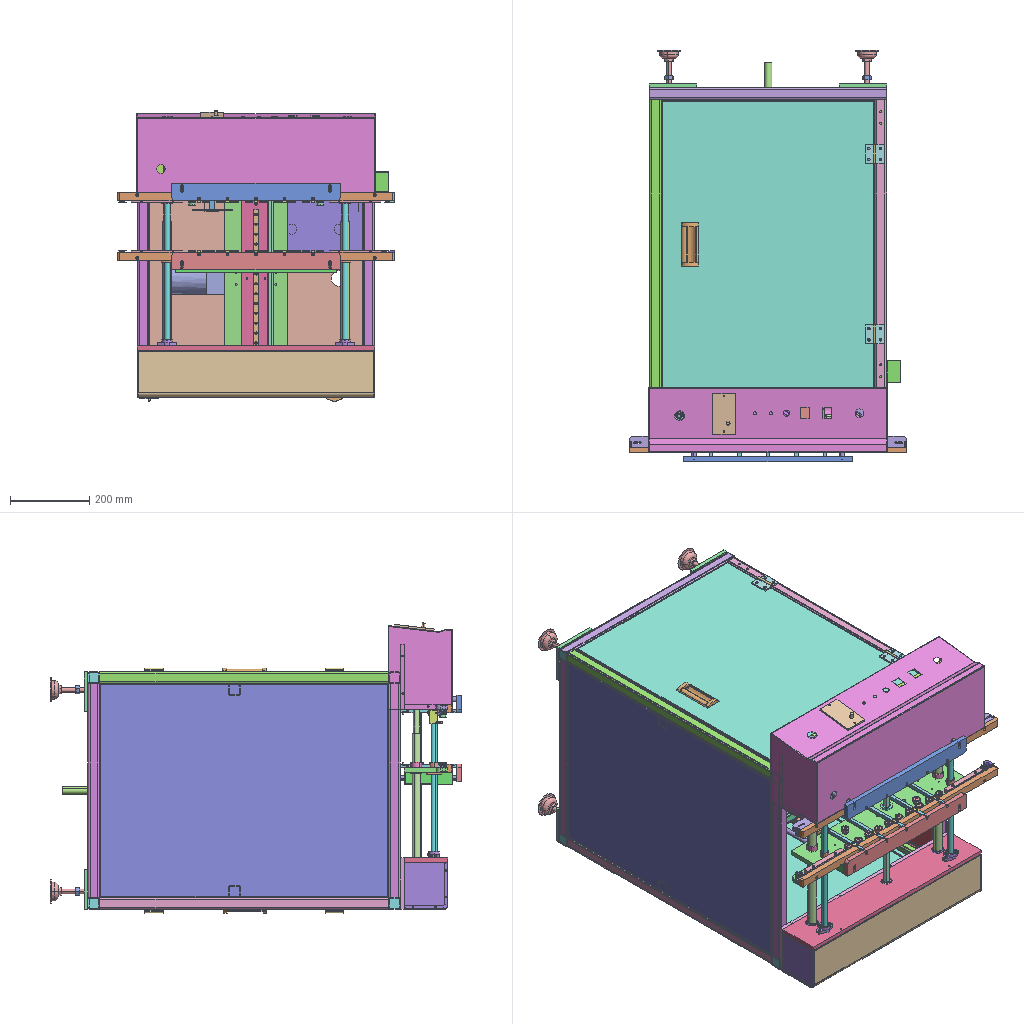Assembly | SolidWorks | 117 different items | 399 placed | box 700 x 1040 x 734 mm
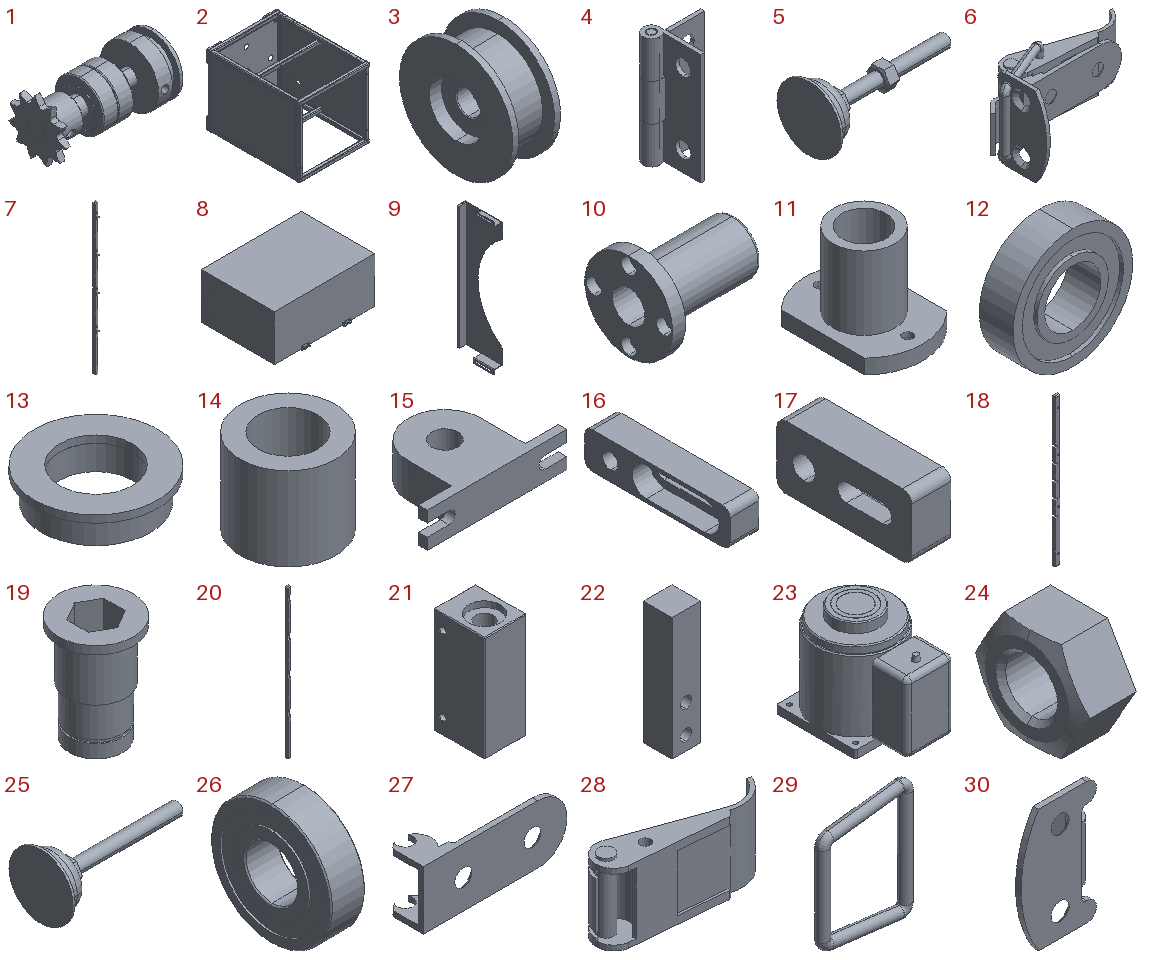Parts list (item | name | quantity | parent item | size | volume | features):
1 | (subassembly) | x22 | - | 38.5 x 19 x 19 mm | 5350 mm3 | -
2 | (subassembly) | x1 | - | 600 x 800 x 600 mm | 4319374 mm3 | -
3 | (subassembly) | x1 | - | 8 x 19 x 19 mm | 1286 mm3 | -
4 | (subassembly) | x2 | in 8 | 11.9 x 11.9 x 25 mm | 590.722 mm3 | -
5 | (subassembly) | x4 | - | 128 x 60 x 60 mm | 51221 mm3 | -
6 | (subassembly) | x2 | in 8 | 39.831 x 19.634 x 22 mm | 1988 mm3 | -
7 | (subassembly) | x10 | - | 8 x 12 x 450 mm | 28666 mm3 | -
8 | (subassembly) | x1 | - | 330 x 252.816 x 156.5 mm | 11874389 mm3 | -
9 | (subassembly) | x1 | - | 21.5 x 91 x 322 mm | 41867 mm3 | -
10 | - | x2 | - | 65 x 54 x 54 mm | 42042 mm3 | features LPattern 1, RevCut 1, Revolution 1
11 | - | x2 | - | 28 x 40 x 30 mm | 8237 mm3 | features ICE 2, Extrusion 1, HoleWzd 1
12 | - | x4 | - | 32 x 9 x 32 mm | 5125 mm3 | features Revolution 1
13 | - | x7 | - | 13.6 x 13.6 x 3.5 mm | 245.378 mm3 | features Extrusion 1, ICE 1
14 | - | x1 | - | 8 x 8 x 7 mm | 214.414 mm3 | features Extrusion 1
15 | - | x2 | - | 80 x 51 x 20 mm | 38253 mm3 | features Extrusion 1, ICE 1
16 | - | x3 | - | 8 x 40 x 10 mm | 1941 mm3 | features Fillet 2, ICE 2, Extrusion 1, HoleWzd 1
17 | - | x1 | - | 8.7 x 30 x 14 mm | 2717 mm3 | features ICE 2, Extrusion 1, Fillet 1, HoleWzd 1
18 | - | x2 | - | 20.5 x 15 x 700 mm | 182437 mm3 | features Chamfer 2, Extrusion 1, Fillet 1, HoleWzd 1, ICE 1
19 | - | x1 | - | 28 x 28 x 39.7 mm | 7720 mm3 | features ICE 5, Extrusion 1, RevCut 1
20 | - | x10 | in 7 | 8 x 8 x 450 mm | 26809 mm3 | features HoleWzd 3, ICE 2, Extrusion 1
21 | - | x4 | - | 28 x 34 x 70 mm | 55264 mm3 | features RevCut 7, ICE 2, Extrusion 1
22 | - | x1 | - | 8 x 8 x 35 mm | 2103 mm3 | features Extrusion 1, HoleWzd 1
23 | - | x2 | - | 80 x 115 x 116 mm | 570040 mm3 | features ICE 7, Fillet 2, 3DProfileFeature 1, Chamfer 1, Extrusion 1, HoleWzd 1
24 | - | x4 | in 5 | 10 x 21.939 x 19 mm | 2247 mm3 | features RefAxis 3, 3DProfileFeature 1, ICE 1, Revolution 1
25 | - | x4 | in 5 | 128 x 60 x 60 mm | 48974 mm3 | features RefAxis 9, 3DProfileFeature 3, ICE 1, Revolution 1
26 | - | x2 | - | 8 x 28 x 28 mm | 3855 mm3 | features RefAxis 3, 3DProfileFeature 1, Revolution 1
27 | - | x2 | in 6 | 27 x 6.688 x 11 mm | 304.183 mm3 | features RefAxis 3, ICE 2, RevCut 2, 3DProfileFeature 1, Extrusion 1
28 | - | x2 | in 6 | 30 x 8.531 x 15 mm | 1203 mm3 | features ICE 6, RefAxis 6, 3DProfileFeature 2, Extrusion 1
29 | - | x2 | in 6 | 16.763 x 2 x 21.5 mm | 200.249 mm3 | features RefAxis 6, Revolution 4, ICE 3, 3DProfileFeature 2, Extrusion 1
30 | - | x2 | in 6 | 13.5 x 6.5 x 22 mm | 280.062 mm3 | features RefAxis 3, ICE 2, RevCut 2, 3DProfileFeature 1, Extrusion 1
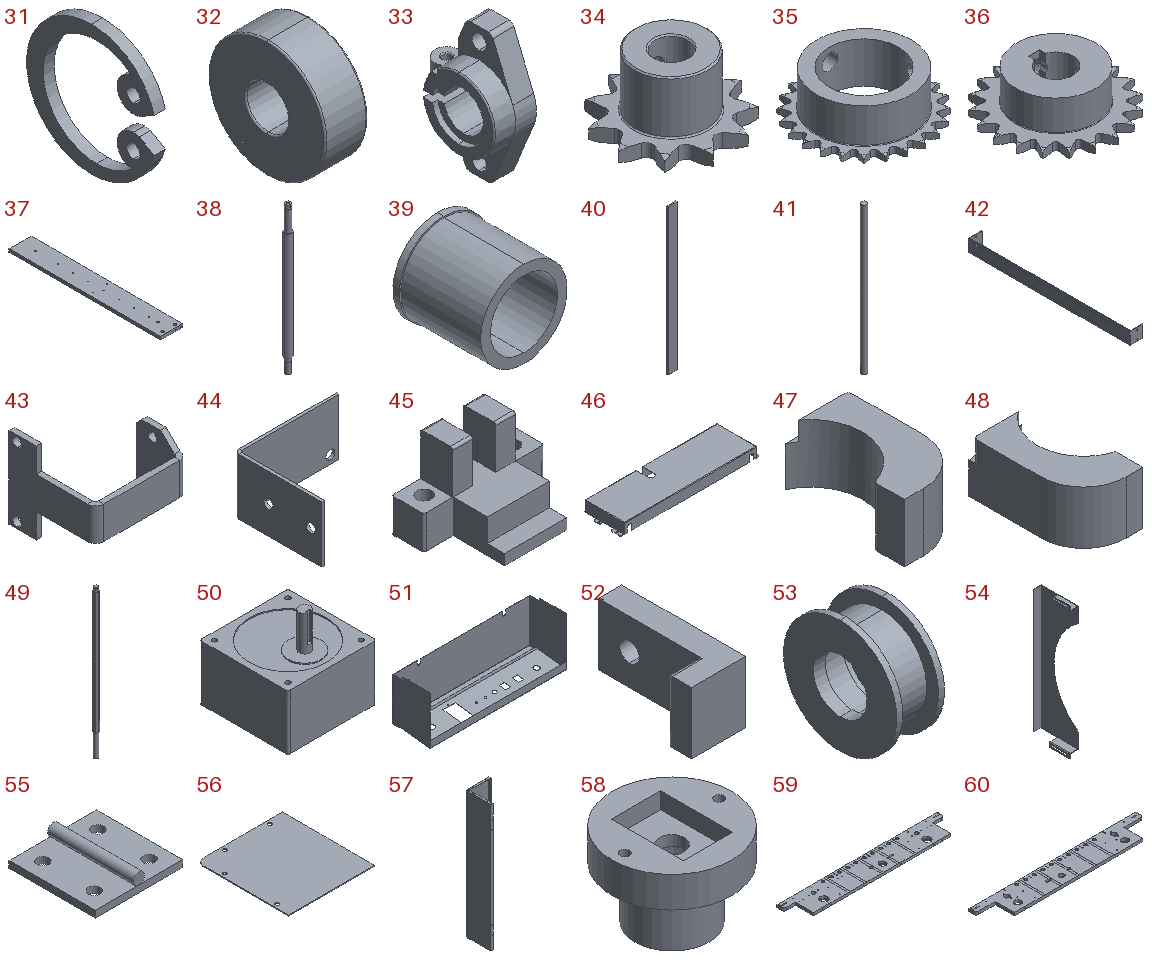31 | - | x1 | in 3 | 1 x 11.586 x 11.8 mm | 42.993 mm3 | features RefAxis 3, 3DProfileFeature 1, Extrusion 1
32 | - | x1 | in 3 | 4 x 11 x 11 mm | 327.696 mm3 | features RefAxis 6, 3DProfileFeature 2, Revolution 1
33 | - | x4 | - | 16 x 31 x 50 mm | 9253 mm3 | features ICE 5, RefAxis 3, RevCut 3, 3DProfileFeature 1, Extrusion 1, Revolution 1
34 | - | x22 | in 1 | 18.807 x 18.615 x 10 mm | 909.903 mm3 | features RevCut 2, ICE 1, Revolution 1
35 | - | x1 | - | 39 x 39 x 13 mm | 4619 mm3 | features ICE 3, RevCut 2, Revolution 1
36 | - | x3 | - | 44 x 44 x 13.5 mm | 8028 mm3 | features ICE 3, RevCut 2, Revolution 1
37 | - | x1 | - | 72 x 496 x 10 mm | 354695 mm3 | features HoleWzd 6, Extrusion 1
38 | - | x2 | - | 21 x 21 x 431 mm | 129224 mm3 | features ICE 5, HoleWzd 2, 3DProfileFeature 1, Extrusion 1
39 | - | x2 | - | 28 x 27 x 28 mm | 6194 mm3 | features Revolution 1
40 | - | x1 | in 9 | 18 x 3 x 300 mm | 16200 mm3 | features Extrusion 1
41 | - | x1 | - | 15 x 15 x 430 mm | 75987 mm3 | features Extrusion 1
42 | - | x1 | - | 31.5 x 395 x 30 mm | 22778 mm3 | features ICE 3, FlatPattern 1, SMBaseFlange 1, SheetMetal 1
43 | - | x1 | - | 34 x 32 x 30 mm | 2372 mm3 | features ICE 5, Chamfer 1, FlatPattern 1, SMBaseFlange 1, SheetMetal 1
44 | - | x3 | - | 36 x 31 x 20 mm | 1279 mm3 | features ICE 2, FlatPattern 1, SMBaseFlange 1, SheetMetal 1
45 | - | x2 | - | 26.2 x 18.3 x 16.6 mm | 2634 mm3 | features ICE 5, Fillet 2, Extrusion 1, MirrorPattern 1
46 | - | x1 | - | 427 x 122 x 32 mm | 79185 mm3 | features Cut 3, EdgeFlange 3, Fillet 1, FlatPattern 1, ICE 1, SMBaseFlange 1, SheetMetal 1
47 | - | x1 | - | 14 x 27 x 12.5 mm | 2830 mm3 | features Fillet 3, Extrusion 1, HoleWzd 1, ICE 1
48 | - | x1 | - | 14 x 27 x 12.5 mm | 2831 mm3 | features Fillet 2, ICE 2, Extrusion 1, HoleWzd 1, MirrorPattern 1
49 | - | x1 | - | 14 x 16.166 x 456 mm | 72301 mm3 | features ICE 3, Fillet 2, Extrusion 1, RevCut 1
50 | - | x2 | - | 80 x 80 x 82 mm | 314622 mm3 | features ICE 5, 3DProfileFeature 1, Extrusion 1, Fillet 1, HoleWzd 1
51 | - | x1 | - | 602 x 163.116 x 210.993 mm | 271035 mm3 | features ICE 6, Cut 3, Fillet 3, ExtruThin 1, MirrorPattern 1
52 | - | x40 | in 7 | 7 x 16 x 8 mm | 464.439 mm3 | features Extrusion 1, Fillet 1, HoleWzd 1
53 | - | x4 | in 3 | 8 x 19 x 19 mm | 915.586 mm3 | features RefAxis 12, 3DProfileFeature 4, Revolution 1
54 | - | x1 | in 9 | 21.5 x 91 x 322 mm | 25667 mm3 | features ICE 3, EdgeFlange 2, FlatPattern 1, SMBaseFlange 1, SheetMetal 1
55 | - | x4 | - | 48 x 47 x 9.7 mm | 9200 mm3 | features Extrusion 1, ICE 1
56 | - | x2 | - | 110 x 118 x 1 mm | 12895 mm3 | features Cut 1, FlatPattern 1, SMBaseFlange 1, SheetMetal 1
57 | - | x1 | - | 110 x 118 x 598 mm | 147295 mm3 | features EdgeFlange 3, ICE 2, FlatPattern 1, HoleWzd 1, SMBaseFlange 1, SheetMetal 1
58 | - | x1 | - | 58 x 58 x 40 mm | 46736 mm3 | features ICE 3, Extrusion 1, HoleWzd 1
59 | - | x1 | - | 700 x 110 x 12 mm | 766656 mm3 | features HoleWzd 15, ICE 11, Cut 1, Extrusion 1, Fillet 1
60 | - | x1 | - | 700 x 110 x 12 mm | 712191 mm3 | features HoleWzd 12, ICE 7, Extrusion 1, Fillet 1, LPattern 1
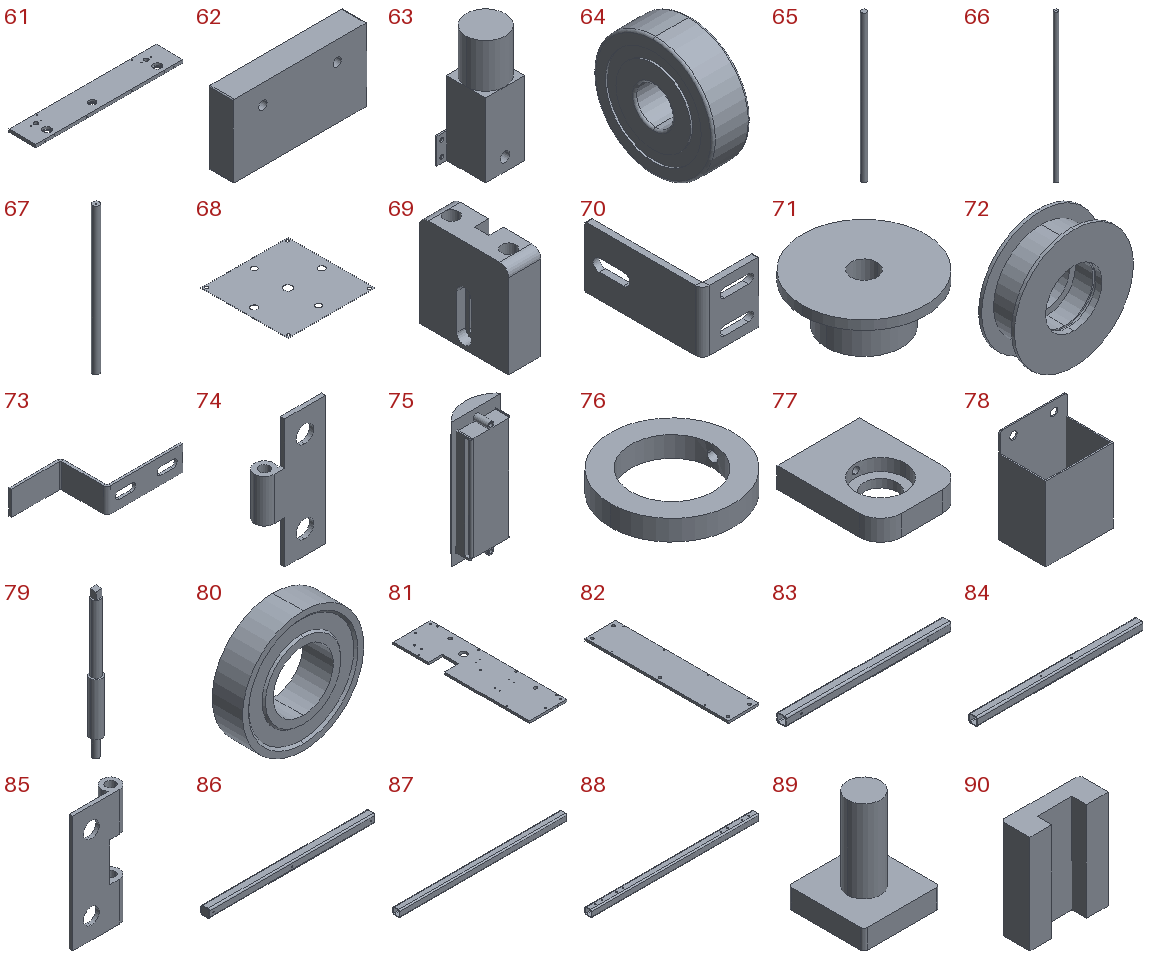61 | - | x1 | - | 600 x 110 x 12 mm | 762368 mm3 | features ICE 5, HoleWzd 4, Extrusion 1
62 | - | x1 | - | 72 x 13 x 39 mm | 36088 mm3 | features Extrusion 1, Fillet 1, ICE 1
63 | - | x1 | - | 120 x 83 x 241 mm | 1411191 mm3 | features ICE 4, Extrusion 1
64 | - | x44 | in 1 | 5 x 16 x 16 mm | 879.517 mm3 | features Revolution 1
65 | - | x2 | - | 15 x 15 x 430 mm | 75987 mm3 | features Extrusion 1
66 | - | x4 | - | 12 x 12 x 448 mm | 50405 mm3 | features HoleWzd 2, Extrusion 1
67 | - | x2 | - | 20 x 20 x 445 mm | 139374 mm3 | features HoleWzd 2, Extrusion 1
68 | - | x1 | in 2 | 540 x 540 x 1 mm | 284181 mm3 | features Cut 2, ICE 2, Extrusion 1
69 | - | x2 | - | 18 x 50 x 52 mm | 37362 mm3 | features ICE 2, Extrusion 1, Fillet 1, HoleWzd 1
70 | - | x1 | - | 28 x 58 x 30 mm | 6672 mm3 | features ICE 2, Fillet 1, FlatPattern 1, SMBaseFlange 1, SheetMetal 1
71 | - | x1 | - | 37.5 x 37.5 x 14.8 mm | 7334 mm3 | features Extrusion 1, ICE 1
72 | - | x4 | - | 40 x 12 x 40 mm | 7443 mm3 | features Revolution 1
73 | - | x1 | - | 51 x 20 x 10 mm | 643.331 mm3 | features EdgeFlange 1, FlatPattern 1, ICE 1, SMBaseFlange 1, SheetMetal 1
74 | - | x2 | in 4 | 11.9 x 3.8 x 25 mm | 218.697 mm3 | features ICE 3, RefAxis 3, 3DProfileFeature 1, Extrusion 1
75 | - | x2 | - | 43.5 x 22.46 x 110 mm | 28533 mm3 | features ICE 3, Extrusion 1, Fillet 1, MirrorPattern 1
76 | - | x1 | - | 30 x 30 x 5 mm | 1939 mm3 | features 3DProfileFeature 1, Extrusion 1, HoleWzd 1
77 | - | x1 | - | 40 x 50 x 10 mm | 15721 mm3 | features HoleWzd 2, ICE 2, Extrusion 1, Fillet 1
78 | - | x1 | - | 50 x 35 x 70 mm | 11415 mm3 | features ICE 3, Extrusion 1, Fillet 1
79 | - | x1 | - | 16 x 16 x 196 mm | 26092 mm3 | features ICE 3, Extrusion 1
80 | - | x1 | - | 24 x 6 x 24 mm | 1915 mm3 | features Revolution 1
81 | - | x1 | - | 165 x 600 x 10 mm | 927945 mm3 | features HoleWzd 8, Cut 2, Extrusion 1, ICE 1
82 | - | x1 | - | 130 x 600 x 10 mm | 774782 mm3 | features HoleWzd 3, Extrusion 1
83 | - | x4 | in 2 | 540 x 30 x 30 mm | 144334 mm3 | features HoleWzd 2, 3DProfileFeature 1, WeldMemberFeat 1, WeldmentFeature 1
84 | - | x2 | in 2 | 598 x 30 x 30 mm | 159852 mm3 | features 3DProfileFeature 1, HoleWzd 1, WeldMemberFeat 1, WeldmentFeature 1
85 | - | x2 | in 4 | 11.9 x 3.8 x 25 mm | 293.72 mm3 | features ICE 3, RefAxis 3, 3DProfileFeature 1, Extrusion 1
86 | - | x4 | in 2 | 600 x 30 x 30 mm | 162072 mm3 | features ICE 2, 3DProfileFeature 1, HoleWzd 1, WeldMemberFeat 1, WeldmentFeature 1
87 | - | x2 | in 2 | 730 x 30 x 30 mm | 195313 mm3 | features 3DProfileFeature 1, WeldMemberFeat 1, WeldmentFeature 1
88 | - | x2 | in 2 | 730 x 30 x 30 mm | 194616 mm3 | features HoleWzd 2, 3DProfileFeature 1, WeldMemberFeat 1, WeldmentFeature 1
89 | - | x1 | - | 23 x 23 x 31 mm | 5132 mm3 | features Extrusion 1, Fillet 1, ICE 1
90 | - | x1 | - | 27 x 10 x 34 mm | 6954 mm3 | features Chamfer 1, Extrusion 1, HoleWzd 1
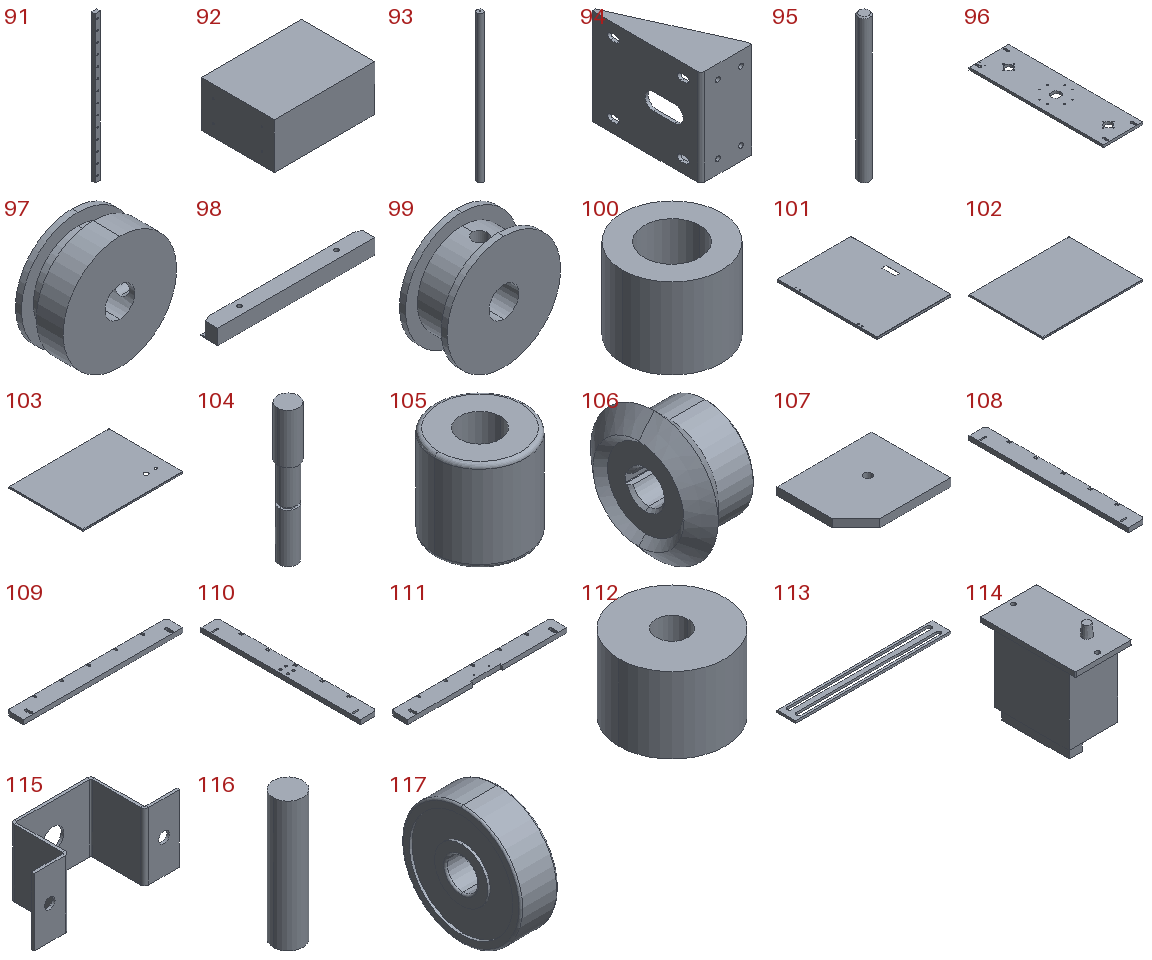91 | - | x1 | - | 12 x 8 x 350 mm | 31582 mm3 | features Chamfer 2, Extrusion 1, HoleWzd 1, LPattern 1
92 | - | x1 | in 8 | 330 x 240 x 150 mm | 11869232 mm3 | features Cut 2, Extrusion 1
93 | - | x1 | - | 20 x 20 x 500 mm | 156724 mm3 | features HoleWzd 2, Extrusion 1
94 | - | x1 | - | 48 x 103 x 91 mm | 51216 mm3 | features ICE 4, Cut 1, FlatPattern 1, SMBaseFlange 1, SheetMetal 1
95 | - | x2 | in 4 | 2 x 2 x 25 mm | 78.305 mm3 | features RefAxis 3, 3DProfileFeature 1, Revolution 1
96 | - | x1 | - | 160 x 540 x 10 mm | 829534 mm3 | features HoleWzd 7, ICE 4, Extrusion 1
97 | - | x22 | in 1 | 19 x 8 x 19 mm | 1809 mm3 | features 3DProfileFeature 1, HoleWzd 1, Revolution 1
98 | - | x4 | - | 130 x 14 x 12.5 mm | 20035 mm3 | features Chamfer 2, Extrusion 1, HoleWzd 1, ICE 1
99 | - | x2 | - | 19 x 8 x 19 mm | 1445 mm3 | features 3DProfileFeature 1, HoleWzd 1, Revolution 1
100 | - | x4 | - | 8 x 8 x 6.5 mm | 223.348 mm3 | features Extrusion 1, ICE 1
101 | - | x2 | - | 539 x 728 x 18 mm | 690643 mm3 | features EdgeFlange 5, Cut 1, FlatPattern 1, ICE 1, SMBaseFlange 1, SheetMetal 1, WeldmentFeature 1
102 | - | x1 | in 2 | 729.5 x 540 x 11.5 mm | 626320 mm3 | features EdgeFlange 3, FlatPattern 1, SMBaseFlange 1, SMMiteredFlange 1, SheetMetal 1
103 | - | x1 | in 2 | 729.5 x 540 x 11.5 mm | 624958 mm3 | features EdgeFlange 3, FlatPattern 1, ICE 1, SMBaseFlange 1, SMMiteredFlange 1, SheetMetal 1
104 | - | x22 | in 1 | 6 x 6 x 38.5 mm | 871.949 mm3 | features Extrusion 1, ICE 1, RevCut 1
105 | - | x2 | - | 45 x 45 x 45 mm | 57194 mm3 | features Extrusion 1, Fillet 1, ICE 1
106 | - | x6 | - | 21.26 x 39.62 x 39.62 mm | 14366 mm3 | features RefAxis 12, 3DProfileFeature 4, RevCut 2, ICE 1, Revolution 1
107 | - | x4 | in 2 | 120 x 100 x 10 mm | 114683 mm3 | features Extrusion 1, HoleWzd 1
108 | - | x1 | - | 44 x 425 x 12 mm | 219705 mm3 | features ICE 5, Extrusion 1, Fillet 1, LPattern 1
109 | - | x1 | - | 425 x 44 x 12 mm | 219705 mm3 | features ICE 5, Extrusion 1, Fillet 1, LPattern 1
110 | - | x1 | - | 44 x 425 x 12 mm | 219009 mm3 | features ICE 5, Extrusion 1, Fillet 1, HoleWzd 1, LPattern 1
111 | - | x1 | - | 425 x 44 x 12 mm | 214700 mm3 | features ICE 6, Extrusion 1, Fillet 1, HoleWzd 1, LPattern 1
112 | - | x4 | - | 14 x 14 x 10 mm | 1401 mm3 | features Extrusion 1, HoleWzd 1
113 | - | x1 | - | 100 x 12 x 1.5 mm | 968.794 mm3 | features Extrusion 1
114 | - | x1 | - | 60 x 102 x 104 mm | 355291 mm3 | features ICE 3, Extrusion 1, Fillet 1
115 | - | x1 | - | 54 x 21 x 25 mm | 2232 mm3 | features ICE 2, FlatPattern 1, SMBaseFlange 1, SheetMetal 1
116 | - | x1 | - | 8 x 8 x 35 mm | 1759 mm3 | features Extrusion 1
117 | - | x4 | - | 6 x 19 x 19 mm | 1455 mm3 | features RefAxis 6, 3DProfileFeature 2, Revolution 1
Mates (type | each side: item.copy, entity, surface, feature), first 403 of 428 lines:
In the top assembly
Coincident | 101.1 face plane Base-Flange 1 | 75.1 face plane Boss-Extrude 1
Coincident | 101.1 face plane Cut-Extrude 1 | 75.1 face plane Boss-Extrude 1
Coincident | 101.1 face plane Cut-Extrude 1 | 75.1 face plane Cut-Extrude 11
Coincident | 101.2 face plane Base-Flange 1 | 75.2 face plane Boss-Extrude 1
Coincident | 101.2 face plane Cut-Extrude 1 | 75.2 face plane Boss-Extrude 1
Coincident | 101.2 face plane Cut-Extrude 1 | 75.2 face plane Cut-Extrude 11
Coincident | 82.1 face plane Boss-Extrude 1 | 59.1 face plane Boss-Extrude 1
Coincident | 59.1 face plane Boss-Extrude 1 | 60.1 face plane Boss-Extrude 1
Coincident | 60.1 face plane Boss-Extrude 1 | 61.1 face plane Boss-Extrude 1
Coincident | 82.1 face plane Boss-Extrude 1 | 61.1 face plane Boss-Extrude 1 | 2 times
Concentric | 60.1 face cylinder Cut-Extrude 2 | 38.1 face cylinder Boss-Extrude 3
Concentric | 59.1 face cylinder Cut-Extrude 3 | 12.1 face cylinder Revolve 1
Coincident | 59.1 face plane Boss-Extrude 1 | 12.1 face plane Revolve 1
Concentric | 59.1 face cylinder Cut-Extrude 3 | 12.2 face cylinder Revolve 1
Coincident | 59.1 face plane Boss-Extrude 1 | 12.2 face plane Revolve 1
Concentric | 38.1 face cylinder Boss-Extrude 3 | 12.3 face cylinder Revolve 1
Coincident | 61.1 face plane Boss-Extrude 1 | 12.3 face plane Revolve 1
Concentric | 61.1 face cylinder Cut-Extrude 2 | 12.4 face cylinder Revolve 1
Coincident | 61.1 face plane Boss-Extrude 1 | 12.4 face plane Revolve 1
Concentric | 60.1 face cylinder Cut-Extrude 2 | 65.1 face cylinder Boss-Extrude 1
Concentric | 60.1 face cylinder Cut-Extrude 2 | 11.1 face cylinder Boss-Extrude 1
Concentric | 65.1 face cylinder Boss-Extrude 1 | 11.2 face cylinder Boss-Extrude 1
Concentric | 12.1 face cylinder Revolve 1 | 38.2 face cylinder Boss-Extrude 1
Concentric | 11.1 face cylinder Boss-Extrude 1 | 65.2 face cylinder Boss-Extrude 1
Coincident | 60.1 face plane Boss-Extrude 1 | 11.1 face plane Boss-Extrude 3
Coincident | 60.1 face plane Boss-Extrude 1 | 11.2 face plane Boss-Extrude 3
Coincident | 61.1 face plane Boss-Extrude 1 | 38.1 face plane Boss-Extrude 3
Concentric | 38.1 face cylinder Boss-Extrude 5 | 36.1 face cylinder Revolve 1
Concentric | 38.2 face cylinder Boss-Extrude 5 | 36.2 face cylinder Revolve 1
Coincident | 61.1 face plane Boss-Extrude 1 | 33.1 face plane Boss-Extrude 1
Concentric | 65.1 face cylinder Boss-Extrude 1 | 33.1 face cylinder Cut-Revolve 1
Coincident | 59.1 face plane Boss-Extrude 1 | 33.2 face plane Boss-Extrude 1
Concentric | 65.1 face cylinder Boss-Extrude 1 | 33.2 face cylinder Cut-Revolve 1
Concentric | 65.2 face cylinder Boss-Extrude 1 | 33.3 face cylinder Cut-Revolve 1
Coincident | 61.1 face plane Boss-Extrude 1 | 33.3 face plane Boss-Extrude 1
Concentric | 65.2 face cylinder Boss-Extrude 1 | 33.4 face cylinder Cut-Revolve 1
Coincident | 59.1 face plane Boss-Extrude 1 | 33.4 face plane Boss-Extrude 1
Concentric | 59.1 face | assembly face | 2 times
Coincident | 59.1 face plane Boss-Extrude 1 | assembly face
Parallel | 61.1 face plane Boss-Extrude 1 | 33.3 face plane Cut-Extrude 2
Parallel | 61.1 face plane Boss-Extrude 1 | 33.1 face plane Cut-Extrude 2
Parallel | 59.1 face plane Boss-Extrude 1 | 33.2 face plane Cut-Extrude 2
Parallel | 59.1 face plane Boss-Extrude 1 | 33.4 face plane Cut-Extrude 2
Concentric | 60.1 face cylinder Cut-Extrude 5 | 53.1 face cylinder Revolve 1
Concentric | 59.1 face cylinder Cut-Extrude 6 | 53.2 face cylinder Revolve 1
Coincident | 60.1 face plane Boss-Extrude 1 | 19.1 face plane Cut-Extrude 1
Coincident | 59.1 face plane Boss-Extrude 1 | 18.1 face plane Boss-Extrude 1 | 3 times
Coincident | 66.1 face plane Boss-Extrude 1 | 66.2 face plane Boss-Extrude 1
Coincident | 66.1 face plane Boss-Extrude 1 | 66.3 face plane Boss-Extrude 1
Coincident | 66.2 face plane Boss-Extrude 1 | 66.4 face plane Boss-Extrude 1
Concentric | 10.1 face cylinder Revolve 1 | 67.1 face cylinder Boss-Extrude 1
Concentric | 10.2 face cylinder Revolve 1 | 67.2 face cylinder Boss-Extrude 1
Concentric | 49.1 face cylinder Boss-Extrude 2 | 106.1 face cylinder Revolve 1
Coincident | 94.1 face plane Base-Flange 1 | 50.1 face plane Boss-Extrude 1
Parallel | 94.1 face plane Base-Flange 1 | 50.1 face plane Boss-Extrude 1
Concentric | 106.2 face cylinder Revolve 1 | 50.1 face cylinder Boss-Extrude 3
Parallel | 81.1 face plane Boss-Extrude 1 | 94.1 face plane Boss-Extrude 2 | 2 times
Coincident | 106.2 face plane Revolve 1 | 50.1 face plane Boss-Extrude 3
Width | 94.1 face plane Boss-Extrude 2 | 94.1 face plane Boss-Extrude 1 | 50.1 face plane Boss-Extrude 1 | 50.1 face plane Boss-Extrude 1
Coincident | 60.1 face plane Boss-Extrude 1 | assembly face
Coincident | 60.1 face plane Boss-Extrude 1 | 18.2 face plane Boss-Extrude 1 | 3 times
Concentric | 49.1 face cylinder Boss-Extrude 2 | 36.3 face cylinder Revolve 1
Concentric | 60.1 face cylinder Cut-Extrude 2 | 35.1 face cylinder Revolve 1
Concentric | 96.1 face cylinder Cut-Extrude 1 | 10.2 face cylinder Revolve 1
Concentric | 96.1 face cylinder Cut-Extrude 1 | 10.1 face cylinder Revolve 1
Parallel | 96.1 face plane Boss-Extrude 1 | 37.1 face plane Boss-Extrude 1
Coincident | 96.1 face plane Boss-Extrude 1 | 10.1 face plane Revolve 1
Coincident | 96.1 face plane Boss-Extrude 1 | 10.2 face plane Revolve 1
Coincident | 37.1 face plane Boss-Extrude 1 | 67.2 face plane Boss-Extrude 1
Coincident | 37.1 face plane Boss-Extrude 1 | 67.1 face plane Boss-Extrude 1
Width | 96.1 face plane Boss-Extrude 1 | 96.1 face plane Boss-Extrude 1 | 37.1 face plane Boss-Extrude 1 | 37.1 face plane Boss-Extrude 1
Coincident | 37.1 face plane Boss-Extrude 1 | 73.1 face plane Base-Flange 1 | 3 times
Coincident | 81.1 face plane Boss-Extrude 1 | 59.1 face plane Boss-Extrude 1 | 2 times
Coincident | 82.1 face plane Boss-Extrude 1 | 57.1 face plane Edge-Flange 1
Coincident | 61.1 face plane Boss-Extrude 1 | 57.1 face plane Edge-Flange 1
Coincident | 57.1 face plane Edge-Flange 2 | 56.1 face plane Base-Flange 1
Coincident | 57.1 face plane Base-Flange 1 | 56.1 face plane Base-Flange 1 | 2 times
Coincident | 57.1 face plane Edge-Flange 3 | 56.2 face plane Base-Flange 1
Coincident | 57.1 face plane Base-Flange 1 | 56.2 face plane Base-Flange 1 | 2 times
Concentric | 53.2 face cylinder Revolve 1 | 100.1 face cylinder Boss-Extrude 1
Coincident | 59.1 face plane Boss-Extrude 1 | 100.1 face plane Boss-Extrude 1
Coincident | 59.1 face plane Boss-Extrude 1 | 44.1 face plane Base-Flange 1
Coincident | 59.1 face plane Boss-Extrude 1 | 44.2 face plane Base-Flange 1
Coincident | 96.1 face plane Boss-Extrude 1 | 42.1 face plane Base-Flange 1 | 2 times
Concentric | 80.1 face cylinder Revolve 1 | 77.1 face cylinder Cut-Extrude 1
Coincident | 80.1 face plane Revolve 1 | 77.1 face plane Boss-Extrude 1
Concentric | 12.1 face cylinder Revolve 1 | 80.1 face cylinder Revolve 1
Concentric | 80.1 face cylinder Revolve 1 | 79.1 face cylinder Boss-Extrude 3
DistanceDim | 77.1 face plane Boss-Extrude 1 | 81.1 face plane Boss-Extrude 1
DistanceDim | 12.1 face plane Revolve 1 | 79.1 face plane Boss-Extrude 3
Concentric | 117.1 face cylinder Revolve 1 | 72.1 face cylinder Revolve 1
Coincident | 117.1 face plane Revolve 1 | 72.1 face plane Revolve 1
Concentric | 72.1 face cylinder Revolve 1 | 112.1 face cylinder Boss-Extrude 1
Coincident | 60.1 face plane Boss-Extrude 1 | 112.1 face plane Boss-Extrude 1
Coincident | 117.1 face plane Revolve 1 | 112.1 face plane Boss-Extrude 1
Concentric | 117.2 face cylinder Revolve 1 | 112.2 face cylinder Boss-Extrude 1
Coincident | 117.2 face plane Revolve 1 | 112.2 face plane Boss-Extrude 1
Concentric | 117.2 face cylinder Revolve 1 | 72.2 face cylinder Revolve 1
Coincident | 60.1 face plane Boss-Extrude 1 | 112.2 face plane Boss-Extrude 1
Concentric | 117.3 face cylinder Revolve 1 | 112.3 face cylinder Boss-Extrude 1
Concentric | 117.3 face cylinder Revolve 1 | 72.3 face cylinder Revolve 1
Coincident | 117.3 face plane Revolve 1 | 72.3 face plane Revolve 1
Coincident | 117.3 face plane Revolve 1 | 112.3 face plane Boss-Extrude 1
Coincident | 59.1 face plane Boss-Extrude 1 | 112.3 face plane Boss-Extrude 1
Concentric | 112.4 face cylinder Boss-Extrude 1 | 72.4 face cylinder Revolve 1
Coincident | 117.2 face plane Revolve 1 | 72.2 face plane Revolve 1
Concentric | 117.4 face cylinder Revolve 1 | 112.4 face cylinder Boss-Extrude 1
Coincident | 117.4 face plane Revolve 1 | 112.4 face plane Boss-Extrude 1
Coincident | 117.4 face plane Revolve 1 | 72.4 face plane Revolve 1
Concentric | 81.1 face cylinder M4 Tapped Hole 1 | 94.1 face cylinder Cut-Extrude 2
DistanceDim | 57.1 face plane Edge-Flange 2 | 82.1 face plane Boss-Extrude 1
Coincident | 59.1 face plane Boss-Extrude 1 | 100.2 face plane Boss-Extrude 1
Concentric | 60.1 face cylinder Cut-Extrude 5 | 100.3 face cylinder Cut-Extrude 1
Coincident | 60.1 face plane Boss-Extrude 1 | 100.3 face plane Boss-Extrude 1
Coincident | 60.1 face plane Boss-Extrude 1 | 46.1 face plane Edge-Flange 1
Width | 60.1 face plane Boss-Extrude 1 | 60.1 face plane Boss-Extrude 1 | 46.1 face plane Edge-Flange 2 | 46.1 face plane Edge-Flange 2
Coincident | 60.1 face plane Boss-Extrude 1 | 46.1 face plane Edge-Flange 3
Concentric | 96.1 face cylinder M5 Tapped Hole 1 | 10.1 face cylinder LPattern 1
Concentric | 96.1 face cylinder M5 Tapped Hole 2 | 10.2 face cylinder LPattern 1
Coincident | 42.1 face plane Base-Flange 1 | 45.1 face plane Boss-Extrude 1
DistanceDim | 45.1 face plane Boss-Extrude 1 | 42.1 face plane Base-Flange 1
DistanceDim | 45.1 face plane Boss-Extrude 1 | 73.1 face plane Edge-Flange 1
Coincident | 42.1 face plane Base-Flange 1 | 45.2 face plane Boss-Extrude 1
Coincident | 45.1 face plane Boss-Extrude 1 | 45.2 face plane Boss-Extrude 1
Coincident | 66.2 face plane Boss-Extrude 1 | 108.1 face plane Boss-Extrude 1
Coincident | 66.4 face plane Boss-Extrude 1 | 109.1 face plane Boss-Extrude 1
Width | 59.1 face plane Boss-Extrude 1 | 59.1 face plane Boss-Extrude 1 | 109.1 face plane Boss-Extrude 1 | 109.1 face plane Boss-Extrude 1
Width | 60.1 face plane Boss-Extrude 1 | 60.1 face plane Boss-Extrude 1 | 108.1 face plane Boss-Extrude 1 | 108.1 face plane Boss-Extrude 1
Width | 59.1 face plane Boss-Extrude 1 | 59.1 face plane Boss-Extrude 1 | 111.1 face plane Boss-Extrude 1 | 111.1 face plane Boss-Extrude 1
Coincident | 59.1 face plane Boss-Extrude 1 | 98.1 face plane Boss-Extrude 1
Parallel | 18.1 face plane Boss-Extrude 1 | 98.1 face plane Boss-Extrude 1
DistanceDim | 98.1 face plane Boss-Extrude 1 | 59.1 face plane Boss-Extrude 1
Coincident | 60.1 face plane Boss-Extrude 1 | 100.4 face plane Boss-Extrude 1
Coincident | 97.1 face plane Revolve 1 | 53.3 face plane Revolve 1
Coincident | 60.1 face plane Boss-Extrude 1 | 98.2 face plane Boss-Extrude 1
DistanceDim | 98.2 face plane Boss-Extrude 1 | 60.1 face plane Boss-Extrude 1
Tangent | 53.1 face cylinder Revolve 1 | 98.2 face plane Cut-Extrude 1
Coincident | 59.1 face plane Boss-Extrude 1 | 98.3 face plane Boss-Extrude 1
DistanceDim | 98.3 face plane Boss-Extrude 1 | 59.1 face plane Boss-Extrude 1
Tangent | 53.4 face cylinder Revolve 1 | 98.3 face plane Cut-Extrude 1
Coincident | 60.1 face plane Boss-Extrude 1 | 98.4 face plane Boss-Extrude 1
DistanceDim | 98.4 face plane Boss-Extrude 1 | 60.1 face plane Boss-Extrude 1
Tangent | 53.3 face cylinder Revolve 1 | 98.4 face plane Cut-Extrude 1
Concentric | 60.1 face cylinder  Drill Hole Size by Socket Head Cap Screw Type 1 | 72.1 face cylinder Revolve 1
Concentric | 60.1 face cylinder Cut-Extrude 7 | 117.2 face cylinder Revolve 1
Concentric | 59.1 face cylinder  Drill Hole Size by Socket Head Cap Screw Type 2 | 117.3 face cylinder Revolve 1
Concentric | 59.1 face cylinder Cut-Extrude 9 | 117.4 face cylinder Revolve 1
Coincident | 59.1 face plane Boss-Extrude 1 | 112.4 face plane Boss-Extrude 1
Width | 36.3 face plane Revolve 1 | 36.3 face plane Revolve 1 | 72.4 face plane Revolve 1 | 72.4 face plane Revolve 1
DistanceDim | 18.1 face plane Boss-Extrude 1 | 44.1 face plane Base-Flange 1
DistanceDim | 18.1 face plane Boss-Extrude 1 | 44.2 face plane Base-Flange 1
Coincident | 59.1 face plane Boss-Extrude 1 | 44.3 face plane Base-Flange 1 | 2 times
DistanceDim | 18.1 face plane Boss-Extrude 1 | 44.3 face plane Base-Flange 1
DistanceDim | 44.2 face plane Base-Flange 1 | 59.1 face plane Boss-Extrude 1
DistanceDim | 44.1 face plane Base-Flange 1 | 59.1 face plane Boss-Extrude 1
Coincident | 23.1 face plane Boss-Extrude 1 | 50.2 face plane Boss-Extrude 1 | 3 times
Coincident | 94.1 face plane Base-Flange 1 | 50.2 face plane Boss-Extrude 1
Width | 94.1 face plane Boss-Extrude 1 | 94.1 face plane Boss-Extrude 2 | 50.2 face plane Boss-Extrude 1 | 50.2 face plane Boss-Extrude 1
Concentric | 106.2 face cylinder Revolve 1 | 50.2 face cylinder Boss-Extrude 3
Coincident | 18.1 face plane Boss-Extrude 1 | 51.1 face plane Extrude- Thin Wall 1
Coincident | 81.1 face plane Boss-Extrude 1 | 51.1 face plane Boss-Extrude 1
Coincident | 59.1 face plane Boss-Extrude 1 | 51.1 face plane Extrude- Thin Wall 1
Coincident | 49.1 face plane Boss-Extrude 2 | 106.1 face plane Revolve 1
DistanceDim | 94.1 face plane Base-Flange 1 | 50.2 face plane Boss-Extrude 1
Coincident | 65.1 face plane Boss-Extrude 1 | 65.2 face plane Boss-Extrude 1
DistanceDim | 65.2 face plane Boss-Extrude 1 | 59.1 face plane Boss-Extrude 1
Concentric | 19.1 face cylinder Cut-Extrude 1 | 76.1 face cylinder Boss-Extrude 1
Coincident | 19.1 face plane Boss-Extrude 3 | 76.1 face plane Boss-Extrude 1
Coincident | 51.1 face plane Extrude- Thin Wall 1 | 114.1 face plane Boss-Extrude 1
DistanceDim | 51.1 edge | 114.1 edge
DistanceDim | 114.1 face plane Boss-Extrude 1 | 51.1 face plane Extrude- Thin Wall 1
Concentric | 35.1 face cylinder Cut-Extrude 3 | 19.1 face cylinder Boss-Extrude 1
Coincident | 96.1 face plane Boss-Extrude 1 | 63.1 face plane Boss-Extrude 2
Concentric | 63.1 face cylinder Cut-Extrude 2 | 93.1 face cylinder Boss-Extrude 1
Concentric | 96.1 face cylinder Cut-Extrude 2 | 93.1 face cylinder Boss-Extrude 1
Parallel | 96.1 face plane Boss-Extrude 1 | 63.1 face plane Boss-Extrude 1
Concentric | 71.1 face cylinder Boss-Extrude 1 | 116.1 face cylinder Boss-Extrude 1
DistanceDim | 71.1 face cylinder Boss-Extrude 1 | 82.1 face plane Boss-Extrude 1
Coincident | 82.1 face plane Boss-Extrude 1 | 69.1 face plane Boss-Extrude 1
Coincident | 82.1 face plane Boss-Extrude 1 | 69.2 face plane Boss-Extrude 1
Coincident | 69.1 face plane Boss-Extrude 1 | 69.2 face plane Boss-Extrude 1
Coincident | 71.1 face plane Boss-Extrude 1 | 69.2 face plane Boss-Extrude 1
Coincident | 116.1 face plane Boss-Extrude 1 | 69.2 face plane Boss-Extrude 1
Coincident | 69.2 face plane Boss-Extrude 1 | 22.1 face plane Boss-Extrude 1 | 2 times
Width | 60.1 face plane Boss-Extrude 1 | 60.1 face plane Boss-Extrude 1 | 54.1 face plane Base-Flange 1 | 54.1 face plane Base-Flange 1
Coincident | 19.1 face plane Boss-Extrude 2 | 54.1 face plane Base-Flange 1
Coincident | 60.1 face plane Boss-Extrude 1 | 17.1 face plane Boss-Extrude 1
Parallel | 18.2 face plane Boss-Extrude 1 | 17.1 face plane Boss-Extrude 1
Coincident | 17.1 face plane Boss-Extrude 1 | 13.1 face plane Boss-Extrude 2
Concentric | 17.1 face cylinder M6 Tapped Hole 1 | 13.1 face cylinder Boss-Extrude 1
Coincident | 82.1 face plane Boss-Extrude 1 | 70.1 face plane Base-Flange 1
Parallel | 82.1 face plane Boss-Extrude 1 | 70.1 face plane Base-Flange 1
Concentric | 67.1 face cylinder Boss-Extrude 1 | 105.1 face cylinder Boss-Extrude 1
Concentric | 67.2 face cylinder Boss-Extrude 1 | 105.2 face cylinder Boss-Extrude 1
Coincident | 10.2 face plane Revolve 1 | 105.2 face plane Boss-Extrude 1
Coincident | 51.1 face plane Boss-Extrude 1 | 78.1 face plane Boss-Extrude 2
Concentric | 93.1 face cylinder Boss-Extrude 1 | 58.1 face cylinder Boss-Extrude 1
Coincident | 60.1 face plane Boss-Extrude 1 | 39.1 face plane Revolve 1
Coincident | 60.1 face plane Boss-Extrude 1 | 39.2 face plane Revolve 1
Concentric | 60.1 face cylinder Cut-Extrude 2 | 39.1 face cylinder Revolve 1
LimitDistanceDim | 109.1 face plane Boss-Extrude 1 | 18.1 face plane Boss-Extrude 1
Concentric | 37.1 face cylinder  Drill Hole Size by Socket Head Cap Screw Type 2 | 67.2 face cylinder Boss-Extrude 1
Coincident | 10.1 face plane Revolve 1 | 105.1 face plane Boss-Extrude 1
Coincident | 110.1 face plane Boss-Extrude 1 | 108.1 face plane Boss-Extrude 1 | 2 times
Coincident | 53.2 face plane Revolve 1 | 98.1 face plane Boss-Extrude 1
Concentric | 66.3 face cylinder Boss-Extrude 1 | 21.1 face cylinder Cut-Revolve 1
Coincident | 59.1 face plane Boss-Extrude 1 | 21.1 face plane Boss-Extrude 1
DistanceDim | 21.1 face plane Boss-Extrude 1 | 81.1 face plane Boss-Extrude 1
Coincident | 59.1 face plane Boss-Extrude 1 | 21.2 face plane Boss-Extrude 1
Concentric | 66.4 face cylinder Boss-Extrude 1 | 21.2 face cylinder Cut-Revolve 1
DistanceDim | 21.2 face plane Boss-Extrude 1 | 81.1 face plane Boss-Extrude 1
DistanceDim | 21.2 face plane Boss-Extrude 1 | 59.1 face plane Boss-Extrude 1
Coincident | 60.1 face plane Boss-Extrude 1 | 21.3 face plane Boss-Extrude 1
Concentric | 66.1 face cylinder Boss-Extrude 1 | 21.3 face cylinder Cut-Revolve 1
DistanceDim | 21.1 face plane Boss-Extrude 1 | 59.1 face plane Boss-Extrude 1
DistanceDim | 21.3 face plane Boss-Extrude 1 | 60.1 face plane Boss-Extrude 1 | 2 times
Coincident | 60.1 face plane Boss-Extrude 1 | 21.4 face plane Boss-Extrude 1
Concentric | 66.2 face cylinder Boss-Extrude 1 | 21.4 face cylinder Cut-Revolve 1
DistanceDim | 21.4 face plane Boss-Extrude 1 | 60.1 face plane Boss-Extrude 1 | 2 times
Coincident | 109.1 face plane Boss-Extrude 1 | 20.1 face plane Boss-Extrude 1
Coincident | 111.1 face plane Boss-Extrude 1 | 20.1 face plane Boss-Extrude 1
Coincident | 108.1 face plane Boss-Extrude 1 | 20.2 face plane Boss-Extrude 1
Coincident | 111.1 face plane Cut-Extrude 4 | 20.1 face plane Boss-Extrude 1
Coincident | 108.1 face plane Cut-Extrude 4 | 20.2 face plane Boss-Extrude 1
Coincident | 53.1 face plane Revolve 1 | 98.2 face plane Boss-Extrude 1
Coincident | 109.1 face plane Cut-Extrude 3 | 20.1 face plane Boss-Extrude 1 | 2 times
Concentric | 60.1 face | assembly face | 2 times
Coincident | 59.1 face plane Cut-Extrude 4 | assembly face
Coincident | 60.1 face plane Cut-Extrude 3 | assembly face
Coincident | 59.1 face plane Cut-Extrude 4 | 64.1 face plane Revolve 1
Coincident | 60.1 face plane Boss-Extrude 1 | 64.2 face plane Revolve 1
Concentric | 49.1 face cylinder Boss-Extrude 3 | 26.1 face cylinder Revolve 1 | 2 times
Coincident | 61.1 face plane Cut-Extrude 3 | 26.1 face plane Revolve 1
Concentric | 49.1 face cylinder Boss-Extrude 2 | 26.2 face cylinder Revolve 1
Coincident | 59.1 face plane Cut-Extrude 7 | 26.2 face plane Revolve 1
Concentric | 59.1 face cylinder Cut-Extrude 13 | 65.1 face cylinder Boss-Extrude 1
Coincident | 37.1 face plane Boss-Extrude 1 | 111.1 face plane Cut-Extrude 3
Concentric | 104.1 face cylinder Boss-Extrude 1 | 99.1 face cylinder Revolve 1
Coincident | 97.2 face plane Revolve 1 | 99.1 face plane Revolve 1
Concentric | 97.3 face cylinder Revolve 1 | 99.2 face cylinder Revolve 1
Coincident | 97.3 face plane Revolve 1 | 99.2 face plane Revolve 1
Coincident | 18.2 face plane Boss-Extrude 1 | 20.2 face plane Boss-Extrude 1
Coincident | 108.1 face plane Cut-Extrude 4 | 20.3 face plane Boss-Extrude 1
Coincident | 34.1 face plane Revolve 1 | 34.2 face plane Revolve 1
Coincident | 34.1 face plane Revolve 1 | 34.3 face plane Revolve 1
Concentric | 61.1 face cylinder Cut-Extrude 3 | 26.1 face cylinder Revolve 1
Coincident | 49.1 face plane Boss-Extrude 1 | 26.1 face plane Revolve 1
Concentric | 38.1 face cylinder Boss-Extrude 3 | 39.2 face cylinder Revolve 1
Coincident | 35.1 face plane Revolve 1 | 34.4 face plane Revolve 1
Coincident | 82.1 face plane Boss-Extrude 1 | 15.1 face plane Boss-Extrude 1
Parallel | 82.1 face plane Boss-Extrude 1 | 15.1 face plane Boss-Extrude 1
Coincident | 82.1 face plane Boss-Extrude 1 | 15.2 face plane Boss-Extrude 1
Coincident | 15.1 face plane Boss-Extrude 1 | 15.2 face plane Boss-Extrude 1
Concentric | 15.1 face cylinder Boss-Extrude 1 | 41.1 face cylinder Boss-Extrude 1
Width | 82.1 face plane Boss-Extrude 1 | 82.1 face plane Boss-Extrude 1 | 41.1 face plane Boss-Extrude 1 | 41.1 face plane Boss-Extrude 1
Coincident | 81.1 face plane Boss-Extrude 1 | 77.1 face plane Boss-Extrude 1
Coincident | 49.1 face plane Boss-Extrude 1 | 19.1 face plane Cut-Extrude 3
Coincident | 38.1 face plane Boss-Extrude 2 | 12.2 face plane Revolve 1
Coincident | 12.1 face plane Revolve 1 | 38.2 face plane Boss-Extrude 2
Concentric | 41.1 face cylinder Boss-Extrude 1 | 106.3 face cylinder Revolve 1
Concentric | 38.1 face cylinder Boss-Extrude 5 | 106.4 face cylinder Revolve 1
Concentric | 38.2 face cylinder Boss-Extrude 5 | 106.5 face cylinder Revolve 1
DistanceDim | 15.1 face plane Boss-Extrude 1 | 82.1 face plane Boss-Extrude 1
Concentric | 41.1 face cylinder Boss-Extrude 1 | 106.6 face cylinder Revolve 1
Concentric | 32.1 face cylinder Revolve 1 | 100.2 face cylinder Boss-Extrude 1
DistanceDim | 100.2 face plane Boss-Extrude 1 | 53.4 face plane Revolve 1
DistanceDim | 18.1 face plane Boss-Extrude 1 | 98.3 face plane Cut-Extrude 1
Coincident | 60.1 face plane Boss-Extrude 1 | 16.1 face plane Boss-Extrude 1
Parallel | 18.2 face plane Boss-Extrude 1 | 16.1 face plane Boss-Extrude 1
Coincident | 13.2 face plane Boss-Extrude 1 | 14.1 face plane Boss-Extrude 1
Concentric | 13.2 face cylinder Boss-Extrude 1 | 14.1 face cylinder Boss-Extrude 1
Concentric | 14.1 face cylinder Boss-Extrude 1 | 13.3 face cylinder Boss-Extrude 1
Coincident | 60.1 face plane Boss-Extrude 1 | 16.2 face plane Boss-Extrude 1
Parallel | 18.2 face plane Boss-Extrude 1 | 16.2 face plane Boss-Extrude 1
Concentric | 37.1 face cylinder M4 Tapped Hole 3 | 58.1 face cylinder  Drill Hole Size by Socket Head Cap Screw Type 1
Coincident | 111.1 face plane Cut-Extrude 3 | 62.1 face plane Boss-Extrude 1
Coincident | 37.1 face plane Boss-Extrude 1 | 62.1 face plane Boss-Extrude 1 | 2 times
Coincident | 111.1 face plane Boss-Extrude 1 | 62.1 face plane Boss-Extrude 1
Coincident | 90.1 face plane Boss-Extrude 1 | 91.1 face plane Boss-Extrude 1 | 2 times
Coincident | 110.1 face plane Cut-Extrude 3 | 20.3 face plane Boss-Extrude 1
Coincident | 37.1 face plane Boss-Extrude 1 | 91.1 face plane Boss-Extrude 1
Width | 37.1 face plane Boss-Extrude 1 | 37.1 face plane Boss-Extrude 1 | 91.1 face plane Boss-Extrude 1 | 91.1 face plane Boss-Extrude 1
Coincident | 110.1 face plane Boss-Extrude 1 | 90.1 face plane Boss-Extrude 1
DistanceDim | 37.1 face plane Boss-Extrude 1 | 91.1 face plane Boss-Extrude 1
Parallel | 60.1 face plane Boss-Extrude 1 | 11.1 face plane Cut-Extrude 1
Parallel | 60.1 face plane Boss-Extrude 1 | 11.2 face plane Cut-Extrude 1
Coincident | 59.1 face plane Boss-Extrude 1 | 47.1 face plane Boss-Extrude 1 | 2 times
Coincident | 18.1 face plane Boss-Extrude 1 | 47.1 face plane Boss-Extrude 1
Coincident | 60.1 face plane Boss-Extrude 1 | 48.1 face plane Boss-Extrude 1
Coincident | 18.2 face plane Boss-Extrude 1 | 48.1 face plane Boss-Extrude 1
Coincident | 60.1 face plane Boss-Extrude 1 | 48.1 face plane Cut-Extrude 2
Concentric | 60.1 face cylinder Cut-Extrude 5 | 53.3 face cylinder Revolve 1
Concentric | 53.3 face cylinder Revolve 1 | 100.4 face cylinder Cut-Extrude 1
Coincident | 92.1 face plane Boss-Extrude 1 | 115.1 face plane Base-Flange 1 | 2 times
Coincident | 113.1 face plane Boss-Extrude 1 | 43.1 face plane Base-Flange 1 | 2 times
Width | 113.1 face plane Boss-Extrude 1 | 113.1 face plane Boss-Extrude 1 | 43.1 face plane Base-Flange 1 | 43.1 face plane Base-Flange 1
Coincident | 44.2 face plane Base-Flange 1 | 43.1 face plane Base-Flange 1
Concentric | 59.1 edge | 43.1 face cylinder Cut-Extrude 1
Parallel | 44.2 face plane Base-Flange 1 | 43.1 face plane Base-Flange 1
Coincident | 84.1 face plane  Structure Member 1 | 96.1 face plane Boss-Extrude 1
Coincident | 84.2 face plane  Structure Member 1 | 96.1 face plane Boss-Extrude 1 | 2 times
Coincident | 88.1 face plane  Structure Member 1 | 101.1 face plane Edge-Flange 3
Coincident | 88.1 face plane  Structure Member 1 | 55.1 face plane Boss-Extrude 1
DistanceDim | 88.1 face plane  Structure Member 1 | 55.1 face cylinder Boss-Extrude 1
Concentric | 88.1 face cylinder M5 Tapped Hole 1 | 55.1 face cylinder Boss-Extrude 1
Concentric | 88.1 face cylinder M5 Tapped Hole 1 | 55.2 face cylinder Boss-Extrude 1
Parallel | 88.1 face plane  Structure Member 1 | 55.2 face plane Boss-Extrude 1
Coincident | 88.1 face plane  Structure Member 1 | 55.2 face plane Boss-Extrude 1
Coincident | 86.1 face plane  Structure Member 1 | 101.2 face plane Edge-Flange 4
Coincident | 86.2 face plane  Structure Member 1 | 82.1 face plane Boss-Extrude 1 | 2 times
Concentric | 107.1 face cylinder M12 Tapped Hole 1 | 25.1 face cylinder Revolve 1
DistanceDim | 25.1 face plane Revolve 1 | 107.1 face plane Boss-Extrude 1
Coincident | 83.1 face plane  Structure Member 1 | 59.1 face plane Boss-Extrude 1
Coincident | 88.2 face plane  Structure Member 1 | 101.2 face plane Edge-Flange 3
Coincident | 88.2 face plane  Structure Member 1 | 55.3 face plane Boss-Extrude 1
Concentric | 88.2 face cylinder M5 Tapped Hole 1 | 55.3 face cylinder Boss-Extrude 1 | 2 times
Coincident | 88.2 face plane  Structure Member 1 | 55.4 face plane Boss-Extrude 1
Concentric | 88.2 face cylinder M5 Tapped Hole 1 | 55.4 face cylinder Boss-Extrude 1 | 2 times
Coincident | 86.3 face plane  Structure Member 1 | 101.1 face plane Edge-Flange 2
Concentric | 107.2 face cylinder M12 Tapped Hole 1 | 25.2 face cylinder Revolve 1
DistanceDim | 107.2 face plane Boss-Extrude 1 | 25.2 face plane Revolve 1
Concentric | 107.3 face cylinder M12 Tapped Hole 1 | 25.3 face cylinder Revolve 1
DistanceDim | 25.3 face plane Revolve 1 | 107.3 face plane Boss-Extrude 1
Concentric | 107.4 face cylinder M12 Tapped Hole 1 | 25.4 face cylinder Revolve 1
DistanceDim | 25.4 face plane Revolve 1 | 107.4 face plane Boss-Extrude 1
Coincident | 83.2 face plane  Structure Member 1 | 82.1 face plane Boss-Extrude 1
Width | 83.2 face plane  Structure Member 1 | 83.1 face plane  Structure Member 1 | 96.1 face plane Boss-Extrude 1 | 96.1 face plane Boss-Extrude 1
Coincident | 101.2 face plane Base-Flange 1 | 88.2 face plane  Structure Member 1
Coincident | 101.1 face plane Base-Flange 1 | 88.1 face plane  Structure Member 1
Coincident | 68.1 face plane Boss-Extrude 1 | 92.1 face plane Boss-Extrude 1
Coincident | 83.3 face plane  Structure Member 1 | 92.1 face plane Boss-Extrude 1
Parallel | 86.4 face plane  Structure Member 1 | 92.1 face plane Boss-Extrude 1
Parallel | 86.2 face plane  Structure Member 1 | 69.1 face plane Boss-Extrude 1
Coincident | 88.2 face plane  Structure Member 1 | 78.1 face plane Boss-Extrude 1
DistanceDim | 83.1 face plane  Structure Member 1 | 15.2 face plane Boss-Extrude 1
DistanceDim | 15.1 face plane Boss-Extrude 1 | 83.2 face plane  Structure Member 1
Coincident | 81.1 face plane Boss-Extrude 1 | 83.1 face plane  Structure Member 1
DistanceDim | 92.1 face plane Boss-Extrude 1 | 86.4 face plane  Structure Member 1
Concentric | 93.1 face cylinder Boss-Extrude 1 | 89.1 face cylinder Boss-Extrude 1
Coincident | 58.1 face plane Cut-Extrude 1 | 89.1 face plane Boss-Extrude 2
Width | 58.1 face plane Cut-Extrude 1 | 58.1 face plane Cut-Extrude 1 | 89.1 face plane Boss-Extrude 2 | 89.1 face plane Boss-Extrude 2
Coincident | 37.1 face plane Boss-Extrude 1 | 58.1 face plane Boss-Extrude 2
Coincident | 93.1 face plane Boss-Extrude 1 | 58.1 face plane Boss-Extrude 3
In subassembly 1
Coincident | 64.3 face plane Revolve 1 | 64.4 face plane Revolve 1
Concentric | 64.3 face cylinder Revolve 1 | 104.2 face cylinder Boss-Extrude 2
Concentric | 64.4 face cylinder Revolve 1 | 104.2 face cylinder Boss-Extrude 1
Concentric | 97.4 face cylinder Revolve 1 | 104.2 face cylinder Boss-Extrude 2
Concentric | 34.5 face cylinder Revolve 1 | 104.2 face cylinder Boss-Extrude 1
Coincident | 97.4 face plane Revolve 1 | 104.2 face plane Boss-Extrude 2
Coincident | 64.3 face plane Revolve 1 | 104.2 face plane Cut-Revolve 1
Coincident | 34.5 face plane Revolve 1 | 104.2 face plane Boss-Extrude 1
In subassembly 7
Coincident | 20.4 face plane Cut-Extrude 2 | 52.1 face plane Boss-Extrude 1 | 2 times
Coincident | 20.4 face plane Boss-Extrude 1 | 52.1 face plane Boss-Extrude 1
Coincident | 20.4 face plane Boss-Extrude 1 | 52.2 face plane Boss-Extrude 1
Coincident | 20.4 face plane Cut-Extrude 3 | 52.2 face plane Boss-Extrude 1 | 2 times
Coincident | 20.4 face plane Boss-Extrude 1 | 52.3 face plane Boss-Extrude 1
Coincident | 20.4 face plane Cut-Extrude 3 | 52.3 face plane Boss-Extrude 1 | 2 times
Coincident | 20.4 face plane Boss-Extrude 1 | 52.4 face plane Boss-Extrude 1
Coincident | 20.4 face plane Cut-Extrude 3 | 52.4 face plane Boss-Extrude 1 | 2 times
In subassembly 9
Coincident | 54.2 face plane Base-Flange 1 | 40.1 face plane Boss-Extrude 1 | 3 times
In subassembly 8
DistanceDim | 92.2 face plane Boss-Extrude 1 | 74.1 face plane Boss-Extrude 1
Coincident | 92.2 face plane Boss-Extrude 1 | 30.1 face plane Boss-Extrude 1
Coincident | 92.2 face plane Boss-Extrude 1 | 27.1 face plane Boss-Extrude 1
Coincident | 92.2 face plane Boss-Extrude 1 | 85.1 face plane Boss-Extrude 1
Coincident | 92.2 face plane Boss-Extrude 1 | 74.2 face plane Boss-Extrude 1
Coincident | 92.2 face plane Boss-Extrude 1 | 85.2 face plane Boss-Extrude 1
Coincident | 92.2 face plane Boss-Extrude 1 | 74.1 face plane Boss-Extrude 1
Coincident | 92.2 face plane Boss-Extrude 1 | 27.2 face plane Boss-Extrude 1
Coincident | 92.2 face plane Boss-Extrude 1 | 30.2 face plane Boss-Extrude 1
In subassembly 6
Coincident | 27.3 plane | 28.1 plane
Coincident | 27.3 axis | 28.1 axis
Coincident | 28.1 plane | 29.1 plane
Coincident | 28.1 axis | 29.1 axis
Coincident | 29.1 plane | 30.3 plane
Coincident | 29.1 axis | 30.3 axis
Perpendicular | 27.3 face plane Boss-Extrude 1 | 30.3 face plane Boss-Extrude 1
In subassembly 4
Coincident | 74.3 plane | 85.3 plane
Coincident | 74.3 axis | 85.3 axis
DistanceDim | 95.1 plane | 74.3 plane
Coincident | 74.3 axis | 95.1 axis | 3 times
PlanarAngleDim | 95.1 plane | 74.3 plane
Perpendicular | 74.3 face plane Boss-Extrude 1 | 85.3 face plane Boss-Extrude 1
In subassembly 2
Coincident | 86.5 face plane  Structure Member 1 | 83.4 face plane  Structure Member 1 | 3 times
Coincident | 83.4 face plane  Structure Member 1 | 107.5 face plane Boss-Extrude 1
Coincident | 83.4 face plane  Structure Member 1 | 107.6 face plane Boss-Extrude 1 | 2 times
Coincident | 86.6 face plane  Structure Member 1 | 83.4 face plane  Structure Member 1
Coincident | 83.4 face plane  Structure Member 1 | 68.2 face plane Boss-Extrude 1
Coincident | 84.3 face plane  Structure Member 1 | 84.4 face plane  Structure Member 1
Coincident | 84.4 face plane  Structure Member 1 | 87.1 face plane  Structure Member 1
Coincident | 86.5 face plane  Structure Member 1 | 68.2 face plane Boss-Extrude 1
Coincident | 83.5 face plane  Structure Member 1 | 102.1 face plane  Miter Flange 1
Coincident | 88.3 face plane  Structure Member 1 | 102.1 face plane Base-Flange 1
Coincident | 87.2 face plane  Structure Member 1 | 102.1 face plane Edge-Flange 1
Coincident | 86.6 face plane  Structure Member 1 | 87.2 face plane  Structure Member 1 | 2 times
Coincident | 86.6 face plane Boss-Extrude 1 | 87.2 face plane  Structure Member 1